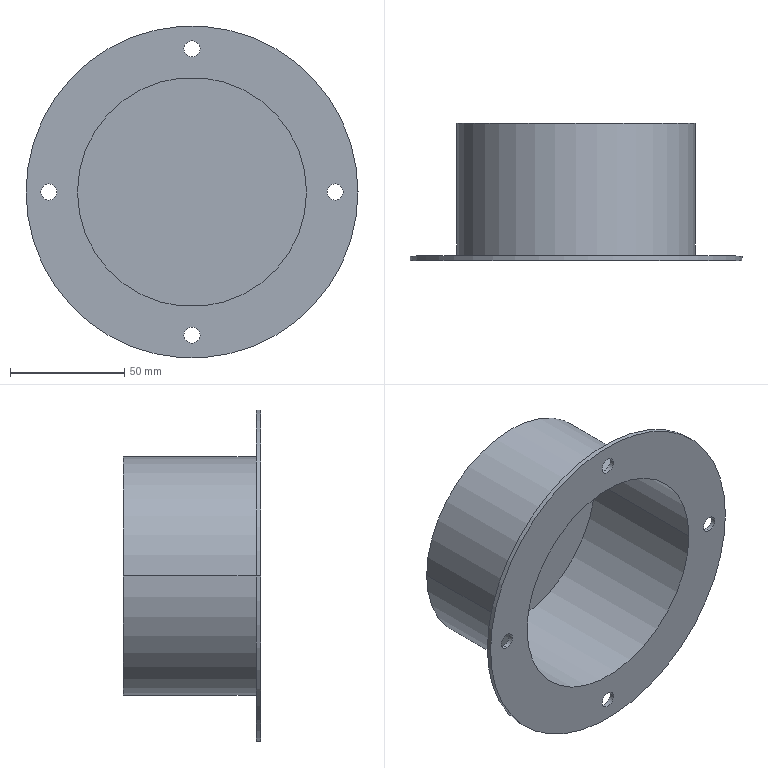Part | SolidWorks | features CirPattern 1, ICE 1, Revolution 1 | 1 solid | 18 faces | box 145 x 60 x 145 mm | volume 69889 mm3 | cylinder 14 | plane 4 | commonest cylinder face diameters 7 x8 100 x2 104 x2 145 x2
STEP:
#1=CARTESIAN_POINT('',(62.5,0.,3.5));
#2=VERTEX_POINT('',#1);
#3=CARTESIAN_POINT('',(62.5,0.,-3.5));
#4=VERTEX_POINT('',#3);
#5=CARTESIAN_POINT('',(62.5,0.,0.));
#6=DIRECTION('',(0.,1.,0.));
#7=DIRECTION('',(0.,0.,-1.));
#8=AXIS2_PLACEMENT_3D('',#5,#6,#7);
#9=CIRCLE('',#8,3.5);
#10=EDGE_CURVE('',#2,#4,#9,.T.);
#11=ORIENTED_EDGE('',*,*,#10,.F.);
#12=CARTESIAN_POINT('',(62.5,2.,3.5));
#13=VERTEX_POINT('',#12);
#14=CARTESIAN_POINT('',(62.5,0.,3.5));
#15=DIRECTION('',(0.,1.,0.));
#16=VECTOR('',#15,1000.);
#17=LINE('',#14,#16);
#18=EDGE_CURVE('',#2,#13,#17,.T.);
#19=ORIENTED_EDGE('',*,*,#18,.T.);
#20=CARTESIAN_POINT('',(62.5,2.,-3.5));
#21=VERTEX_POINT('',#20);
#22=CARTESIAN_POINT('',(62.5,2.,0.));
#23=DIRECTION('',(0.,1.,0.));
#24=DIRECTION('',(0.,0.,-1.));
#25=AXIS2_PLACEMENT_3D('',#22,#23,#24);
#26=CIRCLE('',#25,3.5);
#27=EDGE_CURVE('',#13,#21,#26,.T.);
#28=ORIENTED_EDGE('',*,*,#27,.T.);
#29=CARTESIAN_POINT('',(62.5,0.,-3.5));
#30=DIRECTION('',(0.,1.,0.));
#31=VECTOR('',#30,1000.);
#32=LINE('',#29,#31);
#33=EDGE_CURVE('',#4,#21,#32,.T.);
#34=ORIENTED_EDGE('',*,*,#33,.F.);
#35=EDGE_LOOP('',(#11,#19,#28,#34));
#36=FACE_OUTER_BOUND('',#35,.T.);
#37=CARTESIAN_POINT('',(62.5,0.,0.));
#38=DIRECTION('',(0.,1.,0.));
#39=DIRECTION('',(0.,0.,-1.));
#40=AXIS2_PLACEMENT_3D('',#37,#38,#39);
#41=CYLINDRICAL_SURFACE('',#40,3.5);
#42=ADVANCED_FACE('',(#36),#41,.F.);
#43=CARTESIAN_POINT('',(-3.5,0.,62.5));
#44=VERTEX_POINT('',#43);
#45=CARTESIAN_POINT('',(3.5,0.,62.5));
#46=VERTEX_POINT('',#45);
#47=CARTESIAN_POINT('',(0.,0.,62.5));
#48=DIRECTION('',(0.,1.,0.));
#49=DIRECTION('',(1.,0.,0.));
#50=AXIS2_PLACEMENT_3D('',#47,#48,#49);
#51=CIRCLE('',#50,3.5);
#52=EDGE_CURVE('',#44,#46,#51,.T.);
#53=ORIENTED_EDGE('',*,*,#52,.F.);
#54=CARTESIAN_POINT('',(-3.5,2.,62.5));
#55=VERTEX_POINT('',#54);
#56=CARTESIAN_POINT('',(-3.5,0.,62.5));
#57=DIRECTION('',(0.,1.,0.));
#58=VECTOR('',#57,1000.);
#59=LINE('',#56,#58);
#60=EDGE_CURVE('',#44,#55,#59,.T.);
#61=ORIENTED_EDGE('',*,*,#60,.T.);
#62=CARTESIAN_POINT('',(3.5,2.,62.5));
#63=VERTEX_POINT('',#62);
#64=CARTESIAN_POINT('',(0.,2.,62.5));
#65=DIRECTION('',(0.,1.,0.));
#66=DIRECTION('',(1.,0.,0.));
#67=AXIS2_PLACEMENT_3D('',#64,#65,#66);
#68=CIRCLE('',#67,3.5);
#69=EDGE_CURVE('',#55,#63,#68,.T.);
#70=ORIENTED_EDGE('',*,*,#69,.T.);
#71=CARTESIAN_POINT('',(3.5,0.,62.5));
#72=DIRECTION('',(0.,1.,0.));
#73=VECTOR('',#72,1000.);
#74=LINE('',#71,#73);
#75=EDGE_CURVE('',#46,#63,#74,.T.);
#76=ORIENTED_EDGE('',*,*,#75,.F.);
#77=EDGE_LOOP('',(#53,#61,#70,#76));
#78=FACE_OUTER_BOUND('',#77,.T.);
#79=CARTESIAN_POINT('',(0.,0.,62.5));
#80=DIRECTION('',(0.,1.,0.));
#81=DIRECTION('',(1.,0.,0.));
#82=AXIS2_PLACEMENT_3D('',#79,#80,#81);
#83=CYLINDRICAL_SURFACE('',#82,3.5);
#84=ADVANCED_FACE('',(#78),#83,.F.);
#85=CARTESIAN_POINT('',(-62.5,0.,-3.5));
#86=VERTEX_POINT('',#85);
#87=CARTESIAN_POINT('',(-62.5,0.,3.5));
#88=VERTEX_POINT('',#87);
#89=CARTESIAN_POINT('',(-62.5,0.,0.));
#90=DIRECTION('',(0.,1.,0.));
#91=DIRECTION('',(0.,0.,1.));
#92=AXIS2_PLACEMENT_3D('',#89,#90,#91);
#93=CIRCLE('',#92,3.5);
#94=EDGE_CURVE('',#86,#88,#93,.T.);
#95=ORIENTED_EDGE('',*,*,#94,.F.);
#96=CARTESIAN_POINT('',(-62.5,2.,-3.5));
#97=VERTEX_POINT('',#96);
#98=CARTESIAN_POINT('',(-62.5,0.,-3.5));
#99=DIRECTION('',(0.,1.,0.));
#100=VECTOR('',#99,1000.);
#101=LINE('',#98,#100);
#102=EDGE_CURVE('',#86,#97,#101,.T.);
#103=ORIENTED_EDGE('',*,*,#102,.T.);
#104=CARTESIAN_POINT('',(-62.5,2.,3.5));
#105=VERTEX_POINT('',#104);
#106=CARTESIAN_POINT('',(-62.5,2.,0.));
#107=DIRECTION('',(0.,1.,0.));
#108=DIRECTION('',(0.,0.,1.));
#109=AXIS2_PLACEMENT_3D('',#106,#107,#108);
#110=CIRCLE('',#109,3.5);
#111=EDGE_CURVE('',#97,#105,#110,.T.);
#112=ORIENTED_EDGE('',*,*,#111,.T.);
#113=CARTESIAN_POINT('',(-62.5,0.,3.5));
#114=DIRECTION('',(0.,1.,0.));
#115=VECTOR('',#114,1000.);
#116=LINE('',#113,#115);
#117=EDGE_CURVE('',#88,#105,#116,.T.);
#118=ORIENTED_EDGE('',*,*,#117,.F.);
#119=EDGE_LOOP('',(#95,#103,#112,#118));
#120=FACE_OUTER_BOUND('',#119,.T.);
#121=CARTESIAN_POINT('',(-62.5,0.,0.));
#122=DIRECTION('',(0.,1.,0.));
#123=DIRECTION('',(0.,0.,1.));
#124=AXIS2_PLACEMENT_3D('',#121,#122,#123);
#125=CYLINDRICAL_SURFACE('',#124,3.5);
#126=ADVANCED_FACE('',(#120),#125,.F.);
#127=CARTESIAN_POINT('',(3.5,0.,-62.5));
#128=VERTEX_POINT('',#127);
#129=CARTESIAN_POINT('',(-3.5,0.,-62.5));
#130=VERTEX_POINT('',#129);
#131=CARTESIAN_POINT('',(0.,0.,-62.5));
#132=DIRECTION('',(0.,1.,0.));
#133=DIRECTION('',(-1.,0.,0.));
#134=AXIS2_PLACEMENT_3D('',#131,#132,#133);
#135=CIRCLE('',#134,3.5);
#136=EDGE_CURVE('',#128,#130,#135,.T.);
#137=ORIENTED_EDGE('',*,*,#136,.F.);
#138=CARTESIAN_POINT('',(3.5,2.,-62.5));
#139=VERTEX_POINT('',#138);
#140=CARTESIAN_POINT('',(3.5,0.,-62.5));
#141=DIRECTION('',(0.,1.,0.));
#142=VECTOR('',#141,1000.);
#143=LINE('',#140,#142);
#144=EDGE_CURVE('',#128,#139,#143,.T.);
#145=ORIENTED_EDGE('',*,*,#144,.T.);
#146=CARTESIAN_POINT('',(-3.5,2.,-62.5));
#147=VERTEX_POINT('',#146);
#148=CARTESIAN_POINT('',(0.,2.,-62.5));
#149=DIRECTION('',(0.,1.,0.));
#150=DIRECTION('',(-1.,0.,0.));
#151=AXIS2_PLACEMENT_3D('',#148,#149,#150);
#152=CIRCLE('',#151,3.5);
#153=EDGE_CURVE('',#139,#147,#152,.T.);
#154=ORIENTED_EDGE('',*,*,#153,.T.);
#155=CARTESIAN_POINT('',(-3.5,0.,-62.5));
#156=DIRECTION('',(0.,1.,0.));
#157=VECTOR('',#156,1000.);
#158=LINE('',#155,#157);
#159=EDGE_CURVE('',#130,#147,#158,.T.);
#160=ORIENTED_EDGE('',*,*,#159,.F.);
#161=EDGE_LOOP('',(#137,#145,#154,#160));
#162=FACE_OUTER_BOUND('',#161,.T.);
#163=CARTESIAN_POINT('',(0.,0.,-62.5));
#164=DIRECTION('',(0.,1.,0.));
#165=DIRECTION('',(-1.,0.,0.));
#166=AXIS2_PLACEMENT_3D('',#163,#164,#165);
#167=CYLINDRICAL_SURFACE('',#166,3.5);
#168=ADVANCED_FACE('',(#162),#167,.F.);
#169=CARTESIAN_POINT('',(-52.,2.,0.));
#170=VERTEX_POINT('',#169);
#171=CARTESIAN_POINT('',(52.,2.,0.));
#172=VERTEX_POINT('',#171);
#173=CARTESIAN_POINT('',(0.,2.,0.));
#174=DIRECTION('',(0.,1.,0.));
#175=DIRECTION('',(-1.,0.,0.));
#176=AXIS2_PLACEMENT_3D('',#173,#174,#175);
#177=CIRCLE('',#176,52.);
#178=EDGE_CURVE('',#170,#172,#177,.T.);
#179=ORIENTED_EDGE('',*,*,#178,.T.);
#180=CARTESIAN_POINT('',(52.,60.,0.));
#181=VERTEX_POINT('',#180);
#182=CARTESIAN_POINT('',(52.,60.,0.));
#183=DIRECTION('',(0.,1.,0.));
#184=VECTOR('',#183,1000.);
#185=LINE('',#182,#184);
#186=EDGE_CURVE('',#172,#181,#185,.T.);
#187=ORIENTED_EDGE('',*,*,#186,.T.);
#188=CARTESIAN_POINT('',(-52.,60.,0.));
#189=VERTEX_POINT('',#188);
#190=CARTESIAN_POINT('',(0.,60.,0.));
#191=DIRECTION('',(0.,1.,0.));
#192=DIRECTION('',(-1.,0.,0.));
#193=AXIS2_PLACEMENT_3D('',#190,#191,#192);
#194=CIRCLE('',#193,52.);
#195=EDGE_CURVE('',#189,#181,#194,.T.);
#196=ORIENTED_EDGE('',*,*,#195,.F.);
#197=CARTESIAN_POINT('',(-52.,60.,0.));
#198=DIRECTION('',(0.,1.,0.));
#199=VECTOR('',#198,1000.);
#200=LINE('',#197,#199);
#201=EDGE_CURVE('',#170,#189,#200,.T.);
#202=ORIENTED_EDGE('',*,*,#201,.F.);
#203=EDGE_LOOP('',(#179,#187,#196,#202));
#204=FACE_OUTER_BOUND('',#203,.T.);
#205=CARTESIAN_POINT('',(0.,60.,0.));
#206=DIRECTION('',(0.,1.,0.));
#207=DIRECTION('',(-1.,0.,0.));
#208=AXIS2_PLACEMENT_3D('',#205,#206,#207);
#209=CYLINDRICAL_SURFACE('',#208,52.);
#210=ADVANCED_FACE('',(#204),#209,.T.);
#211=CARTESIAN_POINT('',(-72.5,0.,0.));
#212=VERTEX_POINT('',#211);
#213=CARTESIAN_POINT('',(72.5,0.,0.));
#214=VERTEX_POINT('',#213);
#215=CARTESIAN_POINT('',(0.,0.,0.));
#216=DIRECTION('',(0.,1.,0.));
#217=DIRECTION('',(-1.,0.,0.));
#218=AXIS2_PLACEMENT_3D('',#215,#216,#217);
#219=CIRCLE('',#218,72.5);
#220=EDGE_CURVE('',#212,#214,#219,.T.);
#221=ORIENTED_EDGE('',*,*,#220,.T.);
#222=CARTESIAN_POINT('',(72.5,2.,0.));
#223=VERTEX_POINT('',#222);
#224=CARTESIAN_POINT('',(72.5,60.,0.));
#225=DIRECTION('',(0.,1.,0.));
#226=VECTOR('',#225,1000.);
#227=LINE('',#224,#226);
#228=EDGE_CURVE('',#214,#223,#227,.T.);
#229=ORIENTED_EDGE('',*,*,#228,.T.);
#230=CARTESIAN_POINT('',(-72.5,2.,0.));
#231=VERTEX_POINT('',#230);
#232=CARTESIAN_POINT('',(0.,2.,0.));
#233=DIRECTION('',(0.,1.,0.));
#234=DIRECTION('',(-1.,0.,0.));
#235=AXIS2_PLACEMENT_3D('',#232,#233,#234);
#236=CIRCLE('',#235,72.5);
#237=EDGE_CURVE('',#231,#223,#236,.T.);
#238=ORIENTED_EDGE('',*,*,#237,.F.);
#239=CARTESIAN_POINT('',(-72.5,60.,0.));
#240=DIRECTION('',(0.,1.,0.));
#241=VECTOR('',#240,1000.);
#242=LINE('',#239,#241);
#243=EDGE_CURVE('',#212,#231,#242,.T.);
#244=ORIENTED_EDGE('',*,*,#243,.F.);
#245=EDGE_LOOP('',(#221,#229,#238,#244));
#246=FACE_OUTER_BOUND('',#245,.T.);
#247=CARTESIAN_POINT('',(0.,60.,0.));
#248=DIRECTION('',(0.,1.,0.));
#249=DIRECTION('',(-1.,0.,0.));
#250=AXIS2_PLACEMENT_3D('',#247,#248,#249);
#251=CYLINDRICAL_SURFACE('',#250,72.5);
#252=ADVANCED_FACE('',(#246),#251,.T.);
#253=CARTESIAN_POINT('',(50.,0.,0.));
#254=VERTEX_POINT('',#253);
#255=CARTESIAN_POINT('',(-50.,0.,0.));
#256=VERTEX_POINT('',#255);
#257=CARTESIAN_POINT('',(0.,0.,0.));
#258=DIRECTION('',(0.,1.,0.));
#259=DIRECTION('',(-1.,0.,0.));
#260=AXIS2_PLACEMENT_3D('',#257,#258,#259);
#261=CIRCLE('',#260,50.);
#262=EDGE_CURVE('',#254,#256,#261,.T.);
#263=ORIENTED_EDGE('',*,*,#262,.F.);
#264=CARTESIAN_POINT('',(50.,58.,0.));
#265=VERTEX_POINT('',#264);
#266=CARTESIAN_POINT('',(50.,60.,0.));
#267=DIRECTION('',(0.,1.,0.));
#268=VECTOR('',#267,1000.);
#269=LINE('',#266,#268);
#270=EDGE_CURVE('',#254,#265,#269,.T.);
#271=ORIENTED_EDGE('',*,*,#270,.T.);
#272=CARTESIAN_POINT('',(-50.,58.,0.));
#273=VERTEX_POINT('',#272);
#274=CARTESIAN_POINT('',(0.,58.,0.));
#275=DIRECTION('',(0.,1.,0.));
#276=DIRECTION('',(-1.,0.,0.));
#277=AXIS2_PLACEMENT_3D('',#274,#275,#276);
#278=CIRCLE('',#277,50.);
#279=EDGE_CURVE('',#265,#273,#278,.T.);
#280=ORIENTED_EDGE('',*,*,#279,.T.);
#281=CARTESIAN_POINT('',(-50.,60.,0.));
#282=DIRECTION('',(0.,1.,0.));
#283=VECTOR('',#282,1000.);
#284=LINE('',#281,#283);
#285=EDGE_CURVE('',#256,#273,#284,.T.);
#286=ORIENTED_EDGE('',*,*,#285,.F.);
#287=EDGE_LOOP('',(#263,#271,#280,#286));
#288=FACE_OUTER_BOUND('',#287,.T.);
#289=CARTESIAN_POINT('',(0.,60.,0.));
#290=DIRECTION('',(0.,1.,0.));
#291=DIRECTION('',(-1.,0.,0.));
#292=AXIS2_PLACEMENT_3D('',#289,#290,#291);
#293=CYLINDRICAL_SURFACE('',#292,50.);
#294=ADVANCED_FACE('',(#288),#293,.F.);
#295=ORIENTED_EDGE('',*,*,#270,.F.);
#296=CARTESIAN_POINT('',(0.,0.,0.));
#297=DIRECTION('',(0.,1.,0.));
#298=DIRECTION('',(-1.,0.,0.));
#299=AXIS2_PLACEMENT_3D('',#296,#297,#298);
#300=CIRCLE('',#299,50.);
#301=EDGE_CURVE('',#256,#254,#300,.T.);
#302=ORIENTED_EDGE('',*,*,#301,.F.);
#303=ORIENTED_EDGE('',*,*,#285,.T.);
#304=CARTESIAN_POINT('',(0.,58.,0.));
#305=DIRECTION('',(0.,1.,0.));
#306=DIRECTION('',(-1.,0.,0.));
#307=AXIS2_PLACEMENT_3D('',#304,#305,#306);
#308=CIRCLE('',#307,50.);
#309=EDGE_CURVE('',#273,#265,#308,.T.);
#310=ORIENTED_EDGE('',*,*,#309,.T.);
#311=EDGE_LOOP('',(#295,#302,#303,#310));
#312=FACE_OUTER_BOUND('',#311,.T.);
#313=CARTESIAN_POINT('',(0.,60.,0.));
#314=DIRECTION('',(0.,1.,0.));
#315=DIRECTION('',(-1.,0.,0.));
#316=AXIS2_PLACEMENT_3D('',#313,#314,#315);
#317=CYLINDRICAL_SURFACE('',#316,50.);
#318=ADVANCED_FACE('',(#312),#317,.F.);
#319=CARTESIAN_POINT('',(62.5,0.,0.));
#320=DIRECTION('',(0.,1.,0.));
#321=DIRECTION('',(0.,0.,-1.));
#322=AXIS2_PLACEMENT_3D('',#319,#320,#321);
#323=CIRCLE('',#322,3.5);
#324=EDGE_CURVE('',#4,#2,#323,.T.);
#325=ORIENTED_EDGE('',*,*,#324,.T.);
#326=ORIENTED_EDGE('',*,*,#10,.T.);
#327=EDGE_LOOP('',(#325,#326));
#328=FACE_BOUND('',#327,.T.);
#329=CARTESIAN_POINT('',(0.,0.,62.5));
#330=DIRECTION('',(0.,1.,0.));
#331=DIRECTION('',(1.,0.,0.));
#332=AXIS2_PLACEMENT_3D('',#329,#330,#331);
#333=CIRCLE('',#332,3.5);
#334=EDGE_CURVE('',#46,#44,#333,.T.);
#335=ORIENTED_EDGE('',*,*,#334,.T.);
#336=ORIENTED_EDGE('',*,*,#52,.T.);
#337=EDGE_LOOP('',(#335,#336));
#338=FACE_BOUND('',#337,.T.);
#339=CARTESIAN_POINT('',(-62.5,0.,0.));
#340=DIRECTION('',(0.,1.,0.));
#341=DIRECTION('',(0.,0.,1.));
#342=AXIS2_PLACEMENT_3D('',#339,#340,#341);
#343=CIRCLE('',#342,3.5);
#344=EDGE_CURVE('',#88,#86,#343,.T.);
#345=ORIENTED_EDGE('',*,*,#344,.T.);
#346=ORIENTED_EDGE('',*,*,#94,.T.);
#347=EDGE_LOOP('',(#345,#346));
#348=FACE_BOUND('',#347,.T.);
#349=CARTESIAN_POINT('',(0.,0.,-62.5));
#350=DIRECTION('',(0.,1.,0.));
#351=DIRECTION('',(-1.,0.,0.));
#352=AXIS2_PLACEMENT_3D('',#349,#350,#351);
#353=CIRCLE('',#352,3.5);
#354=EDGE_CURVE('',#130,#128,#353,.T.);
#355=ORIENTED_EDGE('',*,*,#354,.T.);
#356=ORIENTED_EDGE('',*,*,#136,.T.);
#357=EDGE_LOOP('',(#355,#356));
#358=FACE_BOUND('',#357,.T.);
#359=ORIENTED_EDGE('',*,*,#301,.T.);
#360=ORIENTED_EDGE('',*,*,#262,.T.);
#361=EDGE_LOOP('',(#359,#360));
#362=FACE_BOUND('',#361,.T.);
#363=ORIENTED_EDGE('',*,*,#220,.F.);
#364=CARTESIAN_POINT('',(0.,0.,0.));
#365=DIRECTION('',(0.,1.,0.));
#366=DIRECTION('',(-1.,0.,0.));
#367=AXIS2_PLACEMENT_3D('',#364,#365,#366);
#368=CIRCLE('',#367,72.5);
#369=EDGE_CURVE('',#214,#212,#368,.T.);
#370=ORIENTED_EDGE('',*,*,#369,.F.);
#371=EDGE_LOOP('',(#363,#370));
#372=FACE_OUTER_BOUND('',#371,.T.);
#373=CARTESIAN_POINT('',(-50.,0.,0.));
#374=DIRECTION('',(0.,-1.,0.));
#375=DIRECTION('',(1.,0.,0.));
#376=AXIS2_PLACEMENT_3D('',#373,#374,#375);
#377=PLANE('',#376);
#378=ADVANCED_FACE('',(#328,#338,#348,#358,#362,#372),#377,.T.);
#379=ORIENTED_EDGE('',*,*,#228,.F.);
#380=ORIENTED_EDGE('',*,*,#369,.T.);
#381=ORIENTED_EDGE('',*,*,#243,.T.);
#382=CARTESIAN_POINT('',(0.,2.,0.));
#383=DIRECTION('',(0.,1.,0.));
#384=DIRECTION('',(-1.,0.,0.));
#385=AXIS2_PLACEMENT_3D('',#382,#383,#384);
#386=CIRCLE('',#385,72.5);
#387=EDGE_CURVE('',#223,#231,#386,.T.);
#388=ORIENTED_EDGE('',*,*,#387,.F.);
#389=EDGE_LOOP('',(#379,#380,#381,#388));
#390=FACE_OUTER_BOUND('',#389,.T.);
#391=CARTESIAN_POINT('',(0.,60.,0.));
#392=DIRECTION('',(0.,1.,0.));
#393=DIRECTION('',(-1.,0.,0.));
#394=AXIS2_PLACEMENT_3D('',#391,#392,#393);
#395=CYLINDRICAL_SURFACE('',#394,72.5);
#396=ADVANCED_FACE('',(#390),#395,.T.);
#397=CARTESIAN_POINT('',(62.5,2.,0.));
#398=DIRECTION('',(0.,1.,0.));
#399=DIRECTION('',(0.,0.,-1.));
#400=AXIS2_PLACEMENT_3D('',#397,#398,#399);
#401=CIRCLE('',#400,3.5);
#402=EDGE_CURVE('',#21,#13,#401,.T.);
#403=ORIENTED_EDGE('',*,*,#402,.F.);
#404=ORIENTED_EDGE('',*,*,#27,.F.);
#405=EDGE_LOOP('',(#403,#404));
#406=FACE_BOUND('',#405,.T.);
#407=CARTESIAN_POINT('',(0.,2.,62.5));
#408=DIRECTION('',(0.,1.,0.));
#409=DIRECTION('',(1.,0.,0.));
#410=AXIS2_PLACEMENT_3D('',#407,#408,#409);
#411=CIRCLE('',#410,3.5);
#412=EDGE_CURVE('',#63,#55,#411,.T.);
#413=ORIENTED_EDGE('',*,*,#412,.F.);
#414=ORIENTED_EDGE('',*,*,#69,.F.);
#415=EDGE_LOOP('',(#413,#414));
#416=FACE_BOUND('',#415,.T.);
#417=CARTESIAN_POINT('',(-62.5,2.,0.));
#418=DIRECTION('',(0.,1.,0.));
#419=DIRECTION('',(0.,0.,1.));
#420=AXIS2_PLACEMENT_3D('',#417,#418,#419);
#421=CIRCLE('',#420,3.5);
#422=EDGE_CURVE('',#105,#97,#421,.T.);
#423=ORIENTED_EDGE('',*,*,#422,.F.);
#424=ORIENTED_EDGE('',*,*,#111,.F.);
#425=EDGE_LOOP('',(#423,#424));
#426=FACE_BOUND('',#425,.T.);
#427=CARTESIAN_POINT('',(0.,2.,-62.5));
#428=DIRECTION('',(0.,1.,0.));
#429=DIRECTION('',(-1.,0.,0.));
#430=AXIS2_PLACEMENT_3D('',#427,#428,#429);
#431=CIRCLE('',#430,3.5);
#432=EDGE_CURVE('',#147,#139,#431,.T.);
#433=ORIENTED_EDGE('',*,*,#432,.F.);
#434=ORIENTED_EDGE('',*,*,#153,.F.);
#435=EDGE_LOOP('',(#433,#434));
#436=FACE_BOUND('',#435,.T.);
#437=ORIENTED_EDGE('',*,*,#237,.T.);
#438=ORIENTED_EDGE('',*,*,#387,.T.);
#439=EDGE_LOOP('',(#437,#438));
#440=FACE_OUTER_BOUND('',#439,.T.);
#441=ORIENTED_EDGE('',*,*,#178,.F.);
#442=CARTESIAN_POINT('',(0.,2.,0.));
#443=DIRECTION('',(0.,1.,0.));
#444=DIRECTION('',(-1.,0.,0.));
#445=AXIS2_PLACEMENT_3D('',#442,#443,#444);
#446=CIRCLE('',#445,52.);
#447=EDGE_CURVE('',#172,#170,#446,.T.);
#448=ORIENTED_EDGE('',*,*,#447,.F.);
#449=EDGE_LOOP('',(#441,#448));
#450=FACE_BOUND('',#449,.T.);
#451=CARTESIAN_POINT('',(-72.5,2.,0.));
#452=DIRECTION('',(0.,1.,0.));
#453=DIRECTION('',(-1.,0.,0.));
#454=AXIS2_PLACEMENT_3D('',#451,#452,#453);
#455=PLANE('',#454);
#456=ADVANCED_FACE('',(#406,#416,#426,#436,#440,#450),#455,.T.);
#457=ORIENTED_EDGE('',*,*,#186,.F.);
#458=ORIENTED_EDGE('',*,*,#447,.T.);
#459=ORIENTED_EDGE('',*,*,#201,.T.);
#460=CARTESIAN_POINT('',(0.,60.,0.));
#461=DIRECTION('',(0.,1.,0.));
#462=DIRECTION('',(-1.,0.,0.));
#463=AXIS2_PLACEMENT_3D('',#460,#461,#462);
#464=CIRCLE('',#463,52.);
#465=EDGE_CURVE('',#181,#189,#464,.T.);
#466=ORIENTED_EDGE('',*,*,#465,.F.);
#467=EDGE_LOOP('',(#457,#458,#459,#466));
#468=FACE_OUTER_BOUND('',#467,.T.);
#469=CARTESIAN_POINT('',(0.,60.,0.));
#470=DIRECTION('',(0.,1.,0.));
#471=DIRECTION('',(-1.,0.,0.));
#472=AXIS2_PLACEMENT_3D('',#469,#470,#471);
#473=CYLINDRICAL_SURFACE('',#472,52.);
#474=ADVANCED_FACE('',(#468),#473,.T.);
#475=ORIENTED_EDGE('',*,*,#195,.T.);
#476=ORIENTED_EDGE('',*,*,#465,.T.);
#477=EDGE_LOOP('',(#475,#476));
#478=FACE_OUTER_BOUND('',#477,.T.);
#479=CARTESIAN_POINT('',(-52.,60.,0.));
#480=DIRECTION('',(0.,1.,0.));
#481=DIRECTION('',(-1.,0.,0.));
#482=AXIS2_PLACEMENT_3D('',#479,#480,#481);
#483=PLANE('',#482);
#484=ADVANCED_FACE('',(#478),#483,.T.);
#485=ORIENTED_EDGE('',*,*,#309,.F.);
#486=ORIENTED_EDGE('',*,*,#279,.F.);
#487=EDGE_LOOP('',(#485,#486));
#488=FACE_OUTER_BOUND('',#487,.T.);
#489=CARTESIAN_POINT('',(0.,58.,0.));
#490=DIRECTION('',(0.,-1.,0.));
#491=DIRECTION('',(1.,0.,0.));
#492=AXIS2_PLACEMENT_3D('',#489,#490,#491);
#493=PLANE('',#492);
#494=ADVANCED_FACE('',(#488),#493,.T.);
#495=ORIENTED_EDGE('',*,*,#144,.F.);
#496=ORIENTED_EDGE('',*,*,#354,.F.);
#497=ORIENTED_EDGE('',*,*,#159,.T.);
#498=ORIENTED_EDGE('',*,*,#432,.T.);
#499=EDGE_LOOP('',(#495,#496,#497,#498));
#500=FACE_OUTER_BOUND('',#499,.T.);
#501=CARTESIAN_POINT('',(0.,0.,-62.5));
#502=DIRECTION('',(0.,1.,0.));
#503=DIRECTION('',(-1.,0.,0.));
#504=AXIS2_PLACEMENT_3D('',#501,#502,#503);
#505=CYLINDRICAL_SURFACE('',#504,3.5);
#506=ADVANCED_FACE('',(#500),#505,.F.);
#507=ORIENTED_EDGE('',*,*,#102,.F.);
#508=ORIENTED_EDGE('',*,*,#344,.F.);
#509=ORIENTED_EDGE('',*,*,#117,.T.);
#510=ORIENTED_EDGE('',*,*,#422,.T.);
#511=EDGE_LOOP('',(#507,#508,#509,#510));
#512=FACE_OUTER_BOUND('',#511,.T.);
#513=CARTESIAN_POINT('',(-62.5,0.,0.));
#514=DIRECTION('',(0.,1.,0.));
#515=DIRECTION('',(0.,0.,1.));
#516=AXIS2_PLACEMENT_3D('',#513,#514,#515);
#517=CYLINDRICAL_SURFACE('',#516,3.5);
#518=ADVANCED_FACE('',(#512),#517,.F.);
#519=ORIENTED_EDGE('',*,*,#60,.F.);
#520=ORIENTED_EDGE('',*,*,#334,.F.);
#521=ORIENTED_EDGE('',*,*,#75,.T.);
#522=ORIENTED_EDGE('',*,*,#412,.T.);
#523=EDGE_LOOP('',(#519,#520,#521,#522));
#524=FACE_OUTER_BOUND('',#523,.T.);
#525=CARTESIAN_POINT('',(0.,0.,62.5));
#526=DIRECTION('',(0.,1.,0.));
#527=DIRECTION('',(1.,0.,0.));
#528=AXIS2_PLACEMENT_3D('',#525,#526,#527);
#529=CYLINDRICAL_SURFACE('',#528,3.5);
#530=ADVANCED_FACE('',(#524),#529,.F.);
#531=ORIENTED_EDGE('',*,*,#18,.F.);
#532=ORIENTED_EDGE('',*,*,#324,.F.);
#533=ORIENTED_EDGE('',*,*,#33,.T.);
#534=ORIENTED_EDGE('',*,*,#402,.T.);
#535=EDGE_LOOP('',(#531,#532,#533,#534));
#536=FACE_OUTER_BOUND('',#535,.T.);
#537=CARTESIAN_POINT('',(62.5,0.,0.));
#538=DIRECTION('',(0.,1.,0.));
#539=DIRECTION('',(0.,0.,-1.));
#540=AXIS2_PLACEMENT_3D('',#537,#538,#539);
#541=CYLINDRICAL_SURFACE('',#540,3.5);
#542=ADVANCED_FACE('',(#536),#541,.F.);
#543=CLOSED_SHELL('',(#42,#84,#126,#168,#210,#252,#294,#318,#378,#396,#456,#474,#484,#494,#506,#518,#530,#542));
#544=MANIFOLD_SOLID_BREP('',#543);
#545=CARTESIAN_POINT('',(0.,0.,0.));
#546=DIRECTION('',(0.,0.,1.));
#547=DIRECTION('',(1.,0.,0.));
#548=AXIS2_PLACEMENT_3D('',#545,#546,#547);
#549=(LENGTH_UNIT()NAMED_UNIT(*)SI_UNIT(.MILLI.,.METRE.));
#550=UNCERTAINTY_MEASURE_WITH_UNIT(LENGTH_MEASURE(0.00001),#549,'','');
#551=(NAMED_UNIT(*)PLANE_ANGLE_UNIT()SI_UNIT($,.RADIAN.));
#552=(NAMED_UNIT(*)SI_UNIT($,.STERADIAN.)SOLID_ANGLE_UNIT());
#553=(GEOMETRIC_REPRESENTATION_CONTEXT(3)GLOBAL_UNCERTAINTY_ASSIGNED_CONTEXT((#550))GLOBAL_UNIT_ASSIGNED_CONTEXT((#549,#551,#552))REPRESENTATION_CONTEXT('',''));
#554=ADVANCED_BREP_SHAPE_REPRESENTATION('',(#544,#548),#553);